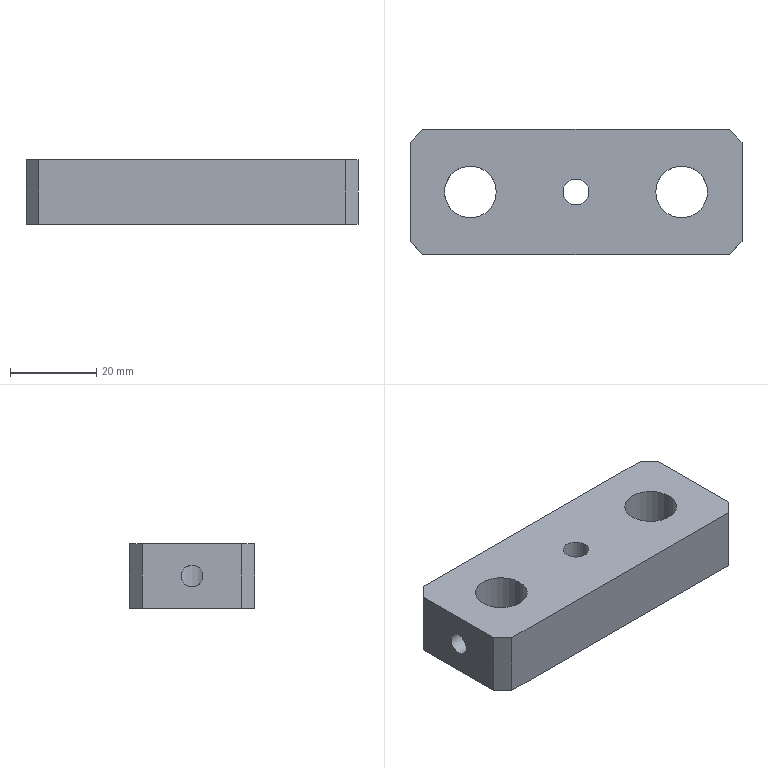Part | NX | features BREP 1 | 1 solid | 17 faces | box 77 x 29 x 15 mm | volume 28818 mm3 | plane 11 | cylinder 6 | commonest cylinder face diameters 5 x2 12 x2 6 x1 8 x1
STEP:
#1=CARTESIAN_POINT('',(-38.5,11.5,15.));
#2=VERTEX_POINT('',#1);
#3=CARTESIAN_POINT('',(-38.5,-11.5,15.));
#4=VERTEX_POINT('',#3);
#5=CARTESIAN_POINT('',(-38.5,0.,15.));
#6=DIRECTION('',(0.,-1.,0.));
#7=VECTOR('',#6,1000.);
#8=LINE('',#5,#7);
#9=EDGE_CURVE('',#2,#4,#8,.T.);
#10=ORIENTED_EDGE('',*,*,#9,.T.);
#11=CARTESIAN_POINT('',(-35.5,-14.5,15.));
#12=VERTEX_POINT('',#11);
#13=CARTESIAN_POINT('',(-38.5,-11.5,15.));
#14=DIRECTION('',(0.7071,-0.7071,0.));
#15=VECTOR('',#14,1000.);
#16=LINE('',#13,#15);
#17=EDGE_CURVE('',#4,#12,#16,.T.);
#18=ORIENTED_EDGE('',*,*,#17,.T.);
#19=CARTESIAN_POINT('',(35.5,-14.5,15.));
#20=VERTEX_POINT('',#19);
#21=CARTESIAN_POINT('',(0.,-14.5,15.));
#22=DIRECTION('',(1.,0.,0.));
#23=VECTOR('',#22,1000.);
#24=LINE('',#21,#23);
#25=EDGE_CURVE('',#12,#20,#24,.T.);
#26=ORIENTED_EDGE('',*,*,#25,.T.);
#27=CARTESIAN_POINT('',(38.5,-11.5,15.));
#28=VERTEX_POINT('',#27);
#29=CARTESIAN_POINT('',(35.5,-14.5,15.));
#30=DIRECTION('',(0.7071,0.7071,0.));
#31=VECTOR('',#30,1000.);
#32=LINE('',#29,#31);
#33=EDGE_CURVE('',#20,#28,#32,.T.);
#34=ORIENTED_EDGE('',*,*,#33,.T.);
#35=CARTESIAN_POINT('',(38.5,11.5,15.));
#36=VERTEX_POINT('',#35);
#37=CARTESIAN_POINT('',(38.5,0.,15.));
#38=DIRECTION('',(0.,1.,0.));
#39=VECTOR('',#38,1000.);
#40=LINE('',#37,#39);
#41=EDGE_CURVE('',#28,#36,#40,.T.);
#42=ORIENTED_EDGE('',*,*,#41,.T.);
#43=CARTESIAN_POINT('',(35.5,14.5,15.));
#44=VERTEX_POINT('',#43);
#45=CARTESIAN_POINT('',(38.5,11.5,15.));
#46=DIRECTION('',(-0.7071,0.7071,0.));
#47=VECTOR('',#46,1000.);
#48=LINE('',#45,#47);
#49=EDGE_CURVE('',#36,#44,#48,.T.);
#50=ORIENTED_EDGE('',*,*,#49,.T.);
#51=CARTESIAN_POINT('',(-35.5,14.5,15.));
#52=VERTEX_POINT('',#51);
#53=CARTESIAN_POINT('',(0.,14.5,15.));
#54=DIRECTION('',(-1.,0.,0.));
#55=VECTOR('',#54,1000.);
#56=LINE('',#53,#55);
#57=EDGE_CURVE('',#44,#52,#56,.T.);
#58=ORIENTED_EDGE('',*,*,#57,.T.);
#59=CARTESIAN_POINT('',(-35.5,14.5,15.));
#60=DIRECTION('',(-0.7071,-0.7071,0.));
#61=VECTOR('',#60,1000.);
#62=LINE('',#59,#61);
#63=EDGE_CURVE('',#52,#2,#62,.T.);
#64=ORIENTED_EDGE('',*,*,#63,.T.);
#65=EDGE_LOOP('',(#10,#18,#26,#34,#42,#50,#58,#64));
#66=FACE_BOUND('',#65,.T.);
#67=CARTESIAN_POINT('',(-18.5,0.,15.));
#68=VERTEX_POINT('',#67);
#69=CARTESIAN_POINT('',(-24.5,0.,15.));
#70=DIRECTION('',(0.,0.,-1.));
#71=DIRECTION('',(1.,0.,0.));
#72=AXIS2_PLACEMENT_3D('',#69,#70,#71);
#73=CIRCLE('',#72,6.);
#74=EDGE_CURVE('',#68,#68,#73,.T.);
#75=ORIENTED_EDGE('',*,*,#74,.T.);
#76=EDGE_LOOP('',(#75));
#77=FACE_BOUND('',#76,.T.);
#78=CARTESIAN_POINT('',(30.5,0.,15.));
#79=VERTEX_POINT('',#78);
#80=CARTESIAN_POINT('',(24.5,0.,15.));
#81=DIRECTION('',(0.,0.,-1.));
#82=DIRECTION('',(1.,0.,0.));
#83=AXIS2_PLACEMENT_3D('',#80,#81,#82);
#84=CIRCLE('',#83,6.);
#85=EDGE_CURVE('',#79,#79,#84,.T.);
#86=ORIENTED_EDGE('',*,*,#85,.T.);
#87=EDGE_LOOP('',(#86));
#88=FACE_BOUND('',#87,.T.);
#89=CARTESIAN_POINT('',(-3.,0.,15.));
#90=VERTEX_POINT('',#89);
#91=CARTESIAN_POINT('',(0.,0.,15.));
#92=DIRECTION('',(0.,0.,-1.));
#93=DIRECTION('',(-1.,0.,0.));
#94=AXIS2_PLACEMENT_3D('',#91,#92,#93);
#95=CIRCLE('',#94,3.);
#96=EDGE_CURVE('',#90,#90,#95,.T.);
#97=ORIENTED_EDGE('',*,*,#96,.T.);
#98=EDGE_LOOP('',(#97));
#99=FACE_BOUND('',#98,.T.);
#100=CARTESIAN_POINT('',(0.,0.,15.));
#101=DIRECTION('',(0.,0.,1.));
#102=DIRECTION('',(-1.,0.,0.));
#103=AXIS2_PLACEMENT_3D('',#100,#101,#102);
#104=PLANE('',#103);
#105=ADVANCED_FACE('',(#66,#77,#88,#99),#104,.T.);
#106=CARTESIAN_POINT('',(-38.5,-11.5,0.));
#107=VERTEX_POINT('',#106);
#108=CARTESIAN_POINT('',(-38.5,-11.5,15.));
#109=DIRECTION('',(0.,0.,1.));
#110=VECTOR('',#109,1000.);
#111=LINE('',#108,#110);
#112=EDGE_CURVE('',#107,#4,#111,.T.);
#113=ORIENTED_EDGE('',*,*,#112,.F.);
#114=CARTESIAN_POINT('',(-35.5,-14.5,0.));
#115=VERTEX_POINT('',#114);
#116=CARTESIAN_POINT('',(-35.5,-14.5,0.));
#117=DIRECTION('',(-0.7071,0.7071,0.));
#118=VECTOR('',#117,1000.);
#119=LINE('',#116,#118);
#120=EDGE_CURVE('',#115,#107,#119,.T.);
#121=ORIENTED_EDGE('',*,*,#120,.F.);
#122=CARTESIAN_POINT('',(-35.5,-14.5,15.));
#123=DIRECTION('',(0.,0.,-1.));
#124=VECTOR('',#123,1000.);
#125=LINE('',#122,#124);
#126=EDGE_CURVE('',#12,#115,#125,.T.);
#127=ORIENTED_EDGE('',*,*,#126,.F.);
#128=ORIENTED_EDGE('',*,*,#17,.F.);
#129=EDGE_LOOP('',(#113,#121,#127,#128));
#130=FACE_BOUND('',#129,.T.);
#131=CARTESIAN_POINT('',(-35.5,-14.5,15.));
#132=DIRECTION('',(0.7071,0.7071,0.));
#133=DIRECTION('',(0.7071,-0.7071,0.));
#134=AXIS2_PLACEMENT_3D('',#131,#132,#133);
#135=PLANE('',#134);
#136=ADVANCED_FACE('',(#130),#135,.F.);
#137=ORIENTED_EDGE('',*,*,#112,.T.);
#138=ORIENTED_EDGE('',*,*,#9,.F.);
#139=CARTESIAN_POINT('',(-38.5,11.5,0.));
#140=VERTEX_POINT('',#139);
#141=CARTESIAN_POINT('',(-38.5,11.5,15.));
#142=DIRECTION('',(0.,0.,1.));
#143=VECTOR('',#142,1000.);
#144=LINE('',#141,#143);
#145=EDGE_CURVE('',#140,#2,#144,.T.);
#146=ORIENTED_EDGE('',*,*,#145,.F.);
#147=CARTESIAN_POINT('',(-38.5,14.5,0.));
#148=DIRECTION('',(0.,1.,0.));
#149=VECTOR('',#148,1000.);
#150=LINE('',#147,#149);
#151=EDGE_CURVE('',#107,#140,#150,.T.);
#152=ORIENTED_EDGE('',*,*,#151,.F.);
#153=EDGE_LOOP('',(#137,#138,#146,#152));
#154=FACE_BOUND('',#153,.T.);
#155=CARTESIAN_POINT('',(-38.5,0.,10.));
#156=VERTEX_POINT('',#155);
#157=CARTESIAN_POINT('',(-38.5,0.,7.5));
#158=DIRECTION('',(-1.,0.,0.));
#159=DIRECTION('',(0.,0.,1.));
#160=AXIS2_PLACEMENT_3D('',#157,#158,#159);
#161=CIRCLE('',#160,2.5);
#162=EDGE_CURVE('',#156,#156,#161,.T.);
#163=ORIENTED_EDGE('',*,*,#162,.F.);
#164=EDGE_LOOP('',(#163));
#165=FACE_BOUND('',#164,.T.);
#166=CARTESIAN_POINT('',(-38.5,14.5,15.));
#167=DIRECTION('',(1.,0.,0.));
#168=DIRECTION('',(0.,0.,1.));
#169=AXIS2_PLACEMENT_3D('',#166,#167,#168);
#170=PLANE('',#169);
#171=ADVANCED_FACE('',(#154,#165),#170,.F.);
#172=CARTESIAN_POINT('',(-35.5,14.5,0.));
#173=VERTEX_POINT('',#172);
#174=CARTESIAN_POINT('',(-35.5,14.5,15.));
#175=DIRECTION('',(0.,0.,1.));
#176=VECTOR('',#175,1000.);
#177=LINE('',#174,#176);
#178=EDGE_CURVE('',#173,#52,#177,.T.);
#179=ORIENTED_EDGE('',*,*,#178,.F.);
#180=CARTESIAN_POINT('',(-38.5,11.5,0.));
#181=DIRECTION('',(0.7071,0.7071,0.));
#182=VECTOR('',#181,1000.);
#183=LINE('',#180,#182);
#184=EDGE_CURVE('',#140,#173,#183,.T.);
#185=ORIENTED_EDGE('',*,*,#184,.F.);
#186=ORIENTED_EDGE('',*,*,#145,.T.);
#187=ORIENTED_EDGE('',*,*,#63,.F.);
#188=EDGE_LOOP('',(#179,#185,#186,#187));
#189=FACE_BOUND('',#188,.T.);
#190=CARTESIAN_POINT('',(-38.5,11.5,15.));
#191=DIRECTION('',(0.7071,-0.7071,0.));
#192=DIRECTION('',(-0.7071,-0.7071,0.));
#193=AXIS2_PLACEMENT_3D('',#190,#191,#192);
#194=PLANE('',#193);
#195=ADVANCED_FACE('',(#189),#194,.F.);
#196=CARTESIAN_POINT('',(35.5,14.5,0.));
#197=VERTEX_POINT('',#196);
#198=CARTESIAN_POINT('',(35.5,14.5,15.));
#199=DIRECTION('',(0.,0.,1.));
#200=VECTOR('',#199,1000.);
#201=LINE('',#198,#200);
#202=EDGE_CURVE('',#197,#44,#201,.T.);
#203=ORIENTED_EDGE('',*,*,#202,.F.);
#204=CARTESIAN_POINT('',(-38.5,14.5,0.));
#205=DIRECTION('',(1.,0.,0.));
#206=VECTOR('',#205,1000.);
#207=LINE('',#204,#206);
#208=EDGE_CURVE('',#173,#197,#207,.T.);
#209=ORIENTED_EDGE('',*,*,#208,.F.);
#210=ORIENTED_EDGE('',*,*,#178,.T.);
#211=ORIENTED_EDGE('',*,*,#57,.F.);
#212=EDGE_LOOP('',(#203,#209,#210,#211));
#213=FACE_BOUND('',#212,.T.);
#214=CARTESIAN_POINT('',(0.,14.5,10.));
#215=VERTEX_POINT('',#214);
#216=CARTESIAN_POINT('',(0.,14.5,7.5));
#217=DIRECTION('',(0.,1.,0.));
#218=DIRECTION('',(0.,0.,1.));
#219=AXIS2_PLACEMENT_3D('',#216,#217,#218);
#220=CIRCLE('',#219,2.5);
#221=EDGE_CURVE('',#215,#215,#220,.T.);
#222=ORIENTED_EDGE('',*,*,#221,.F.);
#223=EDGE_LOOP('',(#222));
#224=FACE_BOUND('',#223,.T.);
#225=CARTESIAN_POINT('',(-38.5,14.5,15.));
#226=DIRECTION('',(0.,-1.,0.));
#227=DIRECTION('',(0.,0.,1.));
#228=AXIS2_PLACEMENT_3D('',#225,#226,#227);
#229=PLANE('',#228);
#230=ADVANCED_FACE('',(#213,#224),#229,.F.);
#231=CARTESIAN_POINT('',(38.5,11.5,0.));
#232=VERTEX_POINT('',#231);
#233=CARTESIAN_POINT('',(38.5,11.5,15.));
#234=DIRECTION('',(0.,0.,1.));
#235=VECTOR('',#234,1000.);
#236=LINE('',#233,#235);
#237=EDGE_CURVE('',#232,#36,#236,.T.);
#238=ORIENTED_EDGE('',*,*,#237,.F.);
#239=CARTESIAN_POINT('',(35.5,14.5,0.));
#240=DIRECTION('',(0.7071,-0.7071,0.));
#241=VECTOR('',#240,1000.);
#242=LINE('',#239,#241);
#243=EDGE_CURVE('',#197,#232,#242,.T.);
#244=ORIENTED_EDGE('',*,*,#243,.F.);
#245=ORIENTED_EDGE('',*,*,#202,.T.);
#246=ORIENTED_EDGE('',*,*,#49,.F.);
#247=EDGE_LOOP('',(#238,#244,#245,#246));
#248=FACE_BOUND('',#247,.T.);
#249=CARTESIAN_POINT('',(35.5,14.5,15.));
#250=DIRECTION('',(-0.7071,-0.7071,0.));
#251=DIRECTION('',(-0.7071,0.7071,0.));
#252=AXIS2_PLACEMENT_3D('',#249,#250,#251);
#253=PLANE('',#252);
#254=ADVANCED_FACE('',(#248),#253,.F.);
#255=CARTESIAN_POINT('',(38.5,-11.5,0.));
#256=VERTEX_POINT('',#255);
#257=CARTESIAN_POINT('',(38.5,-11.5,15.));
#258=DIRECTION('',(0.,0.,1.));
#259=VECTOR('',#258,1000.);
#260=LINE('',#257,#259);
#261=EDGE_CURVE('',#256,#28,#260,.T.);
#262=ORIENTED_EDGE('',*,*,#261,.F.);
#263=CARTESIAN_POINT('',(38.5,14.5,0.));
#264=DIRECTION('',(0.,-1.,0.));
#265=VECTOR('',#264,1000.);
#266=LINE('',#263,#265);
#267=EDGE_CURVE('',#232,#256,#266,.T.);
#268=ORIENTED_EDGE('',*,*,#267,.F.);
#269=ORIENTED_EDGE('',*,*,#237,.T.);
#270=ORIENTED_EDGE('',*,*,#41,.F.);
#271=EDGE_LOOP('',(#262,#268,#269,#270));
#272=FACE_BOUND('',#271,.T.);
#273=CARTESIAN_POINT('',(38.5,14.5,15.));
#274=DIRECTION('',(-1.,0.,0.));
#275=DIRECTION('',(0.,1.,0.));
#276=AXIS2_PLACEMENT_3D('',#273,#274,#275);
#277=PLANE('',#276);
#278=ADVANCED_FACE('',(#272),#277,.F.);
#279=CARTESIAN_POINT('',(35.5,-14.5,0.));
#280=VERTEX_POINT('',#279);
#281=CARTESIAN_POINT('',(35.5,-14.5,15.));
#282=DIRECTION('',(0.,0.,1.));
#283=VECTOR('',#282,1000.);
#284=LINE('',#281,#283);
#285=EDGE_CURVE('',#280,#20,#284,.T.);
#286=ORIENTED_EDGE('',*,*,#285,.F.);
#287=CARTESIAN_POINT('',(38.5,-11.5,0.));
#288=DIRECTION('',(-0.7071,-0.7071,0.));
#289=VECTOR('',#288,1000.);
#290=LINE('',#287,#289);
#291=EDGE_CURVE('',#256,#280,#290,.T.);
#292=ORIENTED_EDGE('',*,*,#291,.F.);
#293=ORIENTED_EDGE('',*,*,#261,.T.);
#294=ORIENTED_EDGE('',*,*,#33,.F.);
#295=EDGE_LOOP('',(#286,#292,#293,#294));
#296=FACE_BOUND('',#295,.T.);
#297=CARTESIAN_POINT('',(38.5,-11.5,15.));
#298=DIRECTION('',(-0.7071,0.7071,0.));
#299=DIRECTION('',(0.7071,0.7071,0.));
#300=AXIS2_PLACEMENT_3D('',#297,#298,#299);
#301=PLANE('',#300);
#302=ADVANCED_FACE('',(#296),#301,.F.);
#303=ORIENTED_EDGE('',*,*,#285,.T.);
#304=ORIENTED_EDGE('',*,*,#25,.F.);
#305=ORIENTED_EDGE('',*,*,#126,.T.);
#306=CARTESIAN_POINT('',(-38.5,-14.5,0.));
#307=DIRECTION('',(-1.,0.,0.));
#308=VECTOR('',#307,1000.);
#309=LINE('',#306,#308);
#310=EDGE_CURVE('',#280,#115,#309,.T.);
#311=ORIENTED_EDGE('',*,*,#310,.F.);
#312=EDGE_LOOP('',(#303,#304,#305,#311));
#313=FACE_BOUND('',#312,.T.);
#314=CARTESIAN_POINT('',(-38.5,-14.5,15.));
#315=DIRECTION('',(0.,1.,0.));
#316=DIRECTION('',(0.,0.,-1.));
#317=AXIS2_PLACEMENT_3D('',#314,#315,#316);
#318=PLANE('',#317);
#319=ADVANCED_FACE('',(#313),#318,.F.);
#320=ORIENTED_EDGE('',*,*,#74,.F.);
#321=EDGE_LOOP('',(#320));
#322=FACE_BOUND('',#321,.T.);
#323=CARTESIAN_POINT('',(-30.5,0.,10.));
#324=VERTEX_POINT('',#323);
#325=CARTESIAN_POINT('',(-30.239,1.962,9.457));
#326=CARTESIAN_POINT('',(-30.63,-0.0004,10.272));
#327=CARTESIAN_POINT('',(-30.24,-1.96,9.456));
#328=CARTESIAN_POINT('',(-29.812,-2.77,7.505));
#329=CARTESIAN_POINT('',(-30.24,-1.959,5.541));
#330=CARTESIAN_POINT('',(-30.63,-0.004978,4.729));
#331=CARTESIAN_POINT('',(-30.24,1.96,5.542));
#332=CARTESIAN_POINT('',(-29.812,2.77,7.497));
#333=CARTESIAN_POINT('',(-30.239,1.962,9.457));
#334=CARTESIAN_POINT('',(-30.63,-0.0004,10.272));
#335=CARTESIAN_POINT('',(-30.24,-1.96,9.456));
#336=B_SPLINE_CURVE_WITH_KNOTS('',3,(#325,#326,#327,#328,#329,#330,#331,#332,#333,#334,#335),.UNSPECIFIED.,.T.,.F.,(1,1,1,1,1,1,1,1,1,1,1,1,1,1,1),(-0.005928,-0.003952,-0.001976,0.,0.001976,0.003952,0.005928,0.007904,0.00988,0.01186,0.01383,0.01581,0.01778,0.01976,0.02174),.UNSPECIFIED.);
#337=EDGE_CURVE('',#324,#324,#336,.T.);
#338=ORIENTED_EDGE('',*,*,#337,.F.);
#339=EDGE_LOOP('',(#338));
#340=FACE_BOUND('',#339,.T.);
#341=CARTESIAN_POINT('',(-18.5,0.,0.));
#342=VERTEX_POINT('',#341);
#343=CARTESIAN_POINT('',(-24.5,0.,0.));
#344=DIRECTION('',(0.,0.,1.));
#345=DIRECTION('',(1.,0.,0.));
#346=AXIS2_PLACEMENT_3D('',#343,#344,#345);
#347=CIRCLE('',#346,6.);
#348=EDGE_CURVE('',#342,#342,#347,.T.);
#349=ORIENTED_EDGE('',*,*,#348,.F.);
#350=EDGE_LOOP('',(#349));
#351=FACE_BOUND('',#350,.T.);
#352=CARTESIAN_POINT('',(-24.5,0.,15.));
#353=DIRECTION('',(0.,0.,1.));
#354=DIRECTION('',(-1.,0.,0.));
#355=AXIS2_PLACEMENT_3D('',#352,#353,#354);
#356=CYLINDRICAL_SURFACE('',#355,6.);
#357=ADVANCED_FACE('',(#322,#340,#351),#356,.F.);
#358=ORIENTED_EDGE('',*,*,#85,.F.);
#359=EDGE_LOOP('',(#358));
#360=FACE_BOUND('',#359,.T.);
#361=CARTESIAN_POINT('',(30.5,0.,0.));
#362=VERTEX_POINT('',#361);
#363=CARTESIAN_POINT('',(24.5,0.,0.));
#364=DIRECTION('',(0.,0.,1.));
#365=DIRECTION('',(1.,0.,0.));
#366=AXIS2_PLACEMENT_3D('',#363,#364,#365);
#367=CIRCLE('',#366,6.);
#368=EDGE_CURVE('',#362,#362,#367,.T.);
#369=ORIENTED_EDGE('',*,*,#368,.F.);
#370=EDGE_LOOP('',(#369));
#371=FACE_BOUND('',#370,.T.);
#372=CARTESIAN_POINT('',(24.5,0.,15.));
#373=DIRECTION('',(0.,0.,1.));
#374=DIRECTION('',(-1.,0.,0.));
#375=AXIS2_PLACEMENT_3D('',#372,#373,#374);
#376=CYLINDRICAL_SURFACE('',#375,6.);
#377=ADVANCED_FACE('',(#360,#371),#376,.F.);
#378=CARTESIAN_POINT('',(-3.,0.,10.));
#379=VERTEX_POINT('',#378);
#380=CARTESIAN_POINT('',(0.,0.,10.));
#381=DIRECTION('',(0.,0.,1.));
#382=DIRECTION('',(-1.,0.,0.));
#383=AXIS2_PLACEMENT_3D('',#380,#381,#382);
#384=CIRCLE('',#383,3.);
#385=EDGE_CURVE('',#379,#379,#384,.T.);
#386=ORIENTED_EDGE('',*,*,#385,.F.);
#387=EDGE_LOOP('',(#386));
#388=FACE_BOUND('',#387,.T.);
#389=ORIENTED_EDGE('',*,*,#96,.F.);
#390=EDGE_LOOP('',(#389));
#391=FACE_BOUND('',#390,.T.);
#392=CARTESIAN_POINT('',(0.,0.,0.));
#393=DIRECTION('',(0.,0.,-1.));
#394=DIRECTION('',(1.,0.,0.));
#395=AXIS2_PLACEMENT_3D('',#392,#393,#394);
#396=CYLINDRICAL_SURFACE('',#395,3.);
#397=ADVANCED_FACE('',(#388,#391),#396,.F.);
#398=ORIENTED_EDGE('',*,*,#291,.T.);
#399=ORIENTED_EDGE('',*,*,#310,.T.);
#400=ORIENTED_EDGE('',*,*,#120,.T.);
#401=ORIENTED_EDGE('',*,*,#151,.T.);
#402=ORIENTED_EDGE('',*,*,#184,.T.);
#403=ORIENTED_EDGE('',*,*,#208,.T.);
#404=ORIENTED_EDGE('',*,*,#243,.T.);
#405=ORIENTED_EDGE('',*,*,#267,.T.);
#406=EDGE_LOOP('',(#398,#399,#400,#401,#402,#403,#404,#405));
#407=FACE_BOUND('',#406,.T.);
#408=ORIENTED_EDGE('',*,*,#348,.T.);
#409=EDGE_LOOP('',(#408));
#410=FACE_BOUND('',#409,.T.);
#411=ORIENTED_EDGE('',*,*,#368,.T.);
#412=EDGE_LOOP('',(#411));
#413=FACE_BOUND('',#412,.T.);
#414=CARTESIAN_POINT('',(-4.,0.,0.));
#415=VERTEX_POINT('',#414);
#416=CARTESIAN_POINT('',(0.,0.,0.));
#417=DIRECTION('',(0.,0.,-1.));
#418=DIRECTION('',(-1.,0.,0.));
#419=AXIS2_PLACEMENT_3D('',#416,#417,#418);
#420=CIRCLE('',#419,4.);
#421=EDGE_CURVE('',#415,#415,#420,.T.);
#422=ORIENTED_EDGE('',*,*,#421,.F.);
#423=EDGE_LOOP('',(#422));
#424=FACE_BOUND('',#423,.T.);
#425=CARTESIAN_POINT('',(0.,0.,0.));
#426=DIRECTION('',(0.,0.,1.));
#427=DIRECTION('',(-1.,0.,0.));
#428=AXIS2_PLACEMENT_3D('',#425,#426,#427);
#429=PLANE('',#428);
#430=ADVANCED_FACE('',(#407,#410,#413,#424),#429,.F.);
#431=ORIENTED_EDGE('',*,*,#337,.T.);
#432=EDGE_LOOP('',(#431));
#433=FACE_BOUND('',#432,.T.);
#434=ORIENTED_EDGE('',*,*,#162,.T.);
#435=EDGE_LOOP('',(#434));
#436=FACE_BOUND('',#435,.T.);
#437=CARTESIAN_POINT('',(-38.5,0.,7.5));
#438=DIRECTION('',(-1.,0.,0.));
#439=DIRECTION('',(0.,0.,-1.));
#440=AXIS2_PLACEMENT_3D('',#437,#438,#439);
#441=CYLINDRICAL_SURFACE('',#440,2.5);
#442=ADVANCED_FACE('',(#433,#436),#441,.F.);
#443=CARTESIAN_POINT('',(0.,4.,10.));
#444=VERTEX_POINT('',#443);
#445=CARTESIAN_POINT('',(-1.967,3.611,9.453));
#446=CARTESIAN_POINT('',(0.001027,4.194,10.273));
#447=CARTESIAN_POINT('',(1.963,3.613,9.453));
#448=CARTESIAN_POINT('',(2.767,2.878,7.507));
#449=CARTESIAN_POINT('',(1.968,3.609,5.551));
#450=CARTESIAN_POINT('',(0.01209,4.194,4.727));
#451=CARTESIAN_POINT('',(-1.961,3.615,5.542));
#452=CARTESIAN_POINT('',(-2.768,2.877,7.492));
#453=CARTESIAN_POINT('',(-1.967,3.611,9.453));
#454=CARTESIAN_POINT('',(0.001027,4.194,10.273));
#455=CARTESIAN_POINT('',(1.963,3.613,9.453));
#456=B_SPLINE_CURVE_WITH_KNOTS('',3,(#445,#446,#447,#448,#449,#450,#451,#452,#453,#454,#455),.UNSPECIFIED.,.T.,.F.,(1,1,1,1,1,1,1,1,1,1,1,1,1,1,1),(-0.006025,-0.004016,-0.002008,0.,0.002008,0.004016,0.006025,0.008033,0.01004,0.01205,0.01406,0.01607,0.01807,0.02008,0.02209),.UNSPECIFIED.);
#457=EDGE_CURVE('',#444,#444,#456,.T.);
#458=ORIENTED_EDGE('',*,*,#457,.F.);
#459=EDGE_LOOP('',(#458));
#460=FACE_BOUND('',#459,.T.);
#461=ORIENTED_EDGE('',*,*,#221,.T.);
#462=EDGE_LOOP('',(#461));
#463=FACE_BOUND('',#462,.T.);
#464=CARTESIAN_POINT('',(0.,14.5,7.5));
#465=DIRECTION('',(0.,1.,0.));
#466=DIRECTION('',(0.,0.,-1.));
#467=AXIS2_PLACEMENT_3D('',#464,#465,#466);
#468=CYLINDRICAL_SURFACE('',#467,2.5);
#469=ADVANCED_FACE('',(#460,#463),#468,.F.);
#470=ORIENTED_EDGE('',*,*,#385,.T.);
#471=EDGE_LOOP('',(#470));
#472=FACE_BOUND('',#471,.T.);
#473=CARTESIAN_POINT('',(0.,0.,10.));
#474=DIRECTION('',(0.,0.,-1.));
#475=DIRECTION('',(-1.,0.,0.));
#476=AXIS2_PLACEMENT_3D('',#473,#474,#475);
#477=CIRCLE('',#476,4.);
#478=EDGE_CURVE('',#444,#444,#477,.T.);
#479=ORIENTED_EDGE('',*,*,#478,.T.);
#480=EDGE_LOOP('',(#479));
#481=FACE_BOUND('',#480,.T.);
#482=CARTESIAN_POINT('',(0.,0.,10.));
#483=DIRECTION('',(0.,0.,-1.));
#484=DIRECTION('',(1.,0.,0.));
#485=AXIS2_PLACEMENT_3D('',#482,#483,#484);
#486=PLANE('',#485);
#487=ADVANCED_FACE('',(#472,#481),#486,.T.);
#488=ORIENTED_EDGE('',*,*,#478,.F.);
#489=ORIENTED_EDGE('',*,*,#457,.T.);
#490=EDGE_LOOP('',(#488,#489));
#491=FACE_BOUND('',#490,.T.);
#492=ORIENTED_EDGE('',*,*,#421,.T.);
#493=EDGE_LOOP('',(#492));
#494=FACE_BOUND('',#493,.T.);
#495=CARTESIAN_POINT('',(0.,0.,10.));
#496=DIRECTION('',(0.,0.,-1.));
#497=DIRECTION('',(1.,0.,0.));
#498=AXIS2_PLACEMENT_3D('',#495,#496,#497);
#499=CYLINDRICAL_SURFACE('',#498,4.);
#500=ADVANCED_FACE('',(#491,#494),#499,.F.);
#501=CLOSED_SHELL('',(#105,#136,#171,#195,#230,#254,#278,#302,#319,#357,#377,#397,#430,#442,#469,#487,#500));
#502=MANIFOLD_SOLID_BREP('',#501);
#503=(LENGTH_UNIT()NAMED_UNIT(*)SI_UNIT(.MILLI.,.METRE.));
#504=UNCERTAINTY_MEASURE_WITH_UNIT(LENGTH_MEASURE(0.0508),#503,'','');
#505=(NAMED_UNIT(*)PLANE_ANGLE_UNIT()SI_UNIT($,.RADIAN.));
#506=(NAMED_UNIT(*)SI_UNIT($,.STERADIAN.)SOLID_ANGLE_UNIT());
#507=(GEOMETRIC_REPRESENTATION_CONTEXT(3)GLOBAL_UNCERTAINTY_ASSIGNED_CONTEXT((#504))GLOBAL_UNIT_ASSIGNED_CONTEXT((#503,#505,#506))REPRESENTATION_CONTEXT('',''));
#508=ADVANCED_BREP_SHAPE_REPRESENTATION('',(#502),#507);